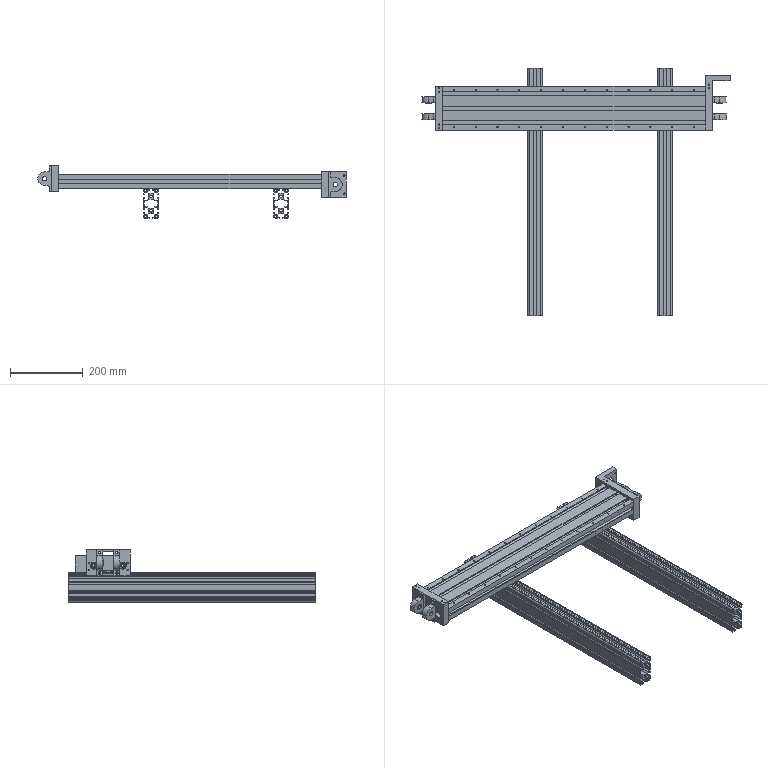Part | 13 solids | 757 faces | box 847 x 680 x 143.5 mm | volume 3322149 mm3 | plane 463 | cylinder 258 | cone 36 | commonest cylinder face diameters 3.3 x128 5 x24 7 x16 12 x16 6.8 x12 9 x10